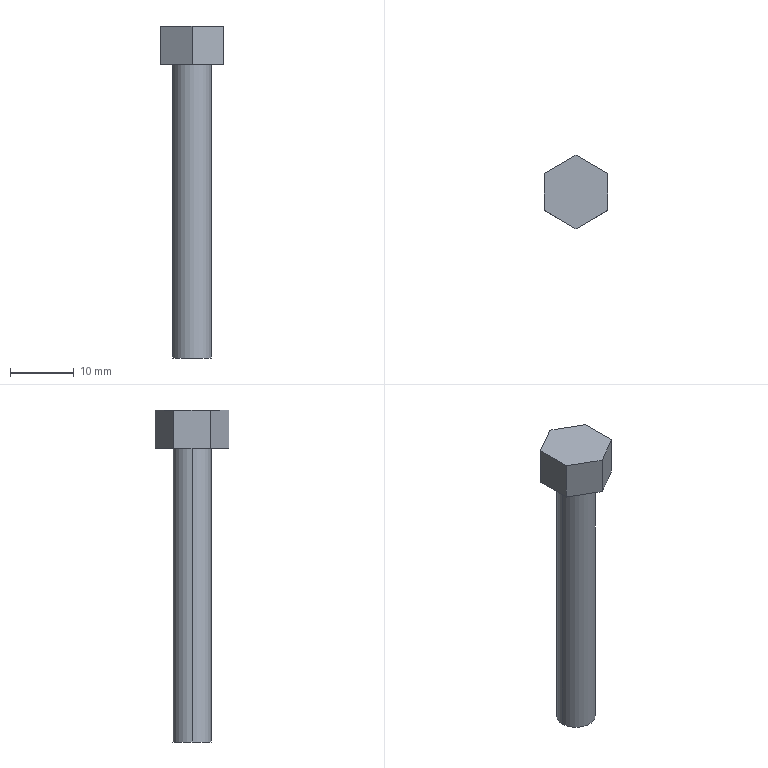Part | STEP file | 11-FG-E00711 | 1 solid | 11 faces | box 10 x 11.547 x 52 mm | volume 1820 mm3 | plane 9 | cylinder 2 | commonest cylinder face diameters 6 x2
STEP:
#1=CARTESIAN_POINT('',(3.,0.,46.));
#2=VERTEX_POINT('',#1);
#3=CARTESIAN_POINT('',(-3.,0.,46.));
#4=VERTEX_POINT('',#3);
#5=CARTESIAN_POINT('',(0.,0.,46.));
#6=DIRECTION('',(0.,0.,1.));
#7=DIRECTION('',(1.,0.,0.));
#8=AXIS2_PLACEMENT_3D('',#5,#6,#7);
#9=CIRCLE('',#8,3.);
#10=EDGE_CURVE('',#2,#4,#9,.T.);
#11=ORIENTED_EDGE('',*,*,#10,.F.);
#12=CARTESIAN_POINT('',(3.,0.,0.));
#13=VERTEX_POINT('',#12);
#14=CARTESIAN_POINT('',(3.,0.,46.));
#15=DIRECTION('',(0.,0.,-1.));
#16=VECTOR('',#15,1000.);
#17=LINE('',#14,#16);
#18=EDGE_CURVE('',#2,#13,#17,.T.);
#19=ORIENTED_EDGE('',*,*,#18,.T.);
#20=CARTESIAN_POINT('',(-3.,0.,0.));
#21=VERTEX_POINT('',#20);
#22=CARTESIAN_POINT('',(0.,0.,0.));
#23=DIRECTION('',(0.,0.,1.));
#24=DIRECTION('',(1.,0.,0.));
#25=AXIS2_PLACEMENT_3D('',#22,#23,#24);
#26=CIRCLE('',#25,3.);
#27=EDGE_CURVE('',#13,#21,#26,.T.);
#28=ORIENTED_EDGE('',*,*,#27,.T.);
#29=CARTESIAN_POINT('',(-3.,0.,46.));
#30=DIRECTION('',(0.,0.,-1.));
#31=VECTOR('',#30,1000.);
#32=LINE('',#29,#31);
#33=EDGE_CURVE('',#4,#21,#32,.T.);
#34=ORIENTED_EDGE('',*,*,#33,.F.);
#35=EDGE_LOOP('',(#11,#19,#28,#34));
#36=FACE_OUTER_BOUND('',#35,.T.);
#37=CARTESIAN_POINT('',(0.,0.,46.));
#38=DIRECTION('',(0.,0.,-1.));
#39=DIRECTION('',(-1.,0.,0.));
#40=AXIS2_PLACEMENT_3D('',#37,#38,#39);
#41=CYLINDRICAL_SURFACE('',#40,3.);
#42=ADVANCED_FACE('',(#36),#41,.T.);
#43=ORIENTED_EDGE('',*,*,#18,.F.);
#44=CARTESIAN_POINT('',(0.,0.,46.));
#45=DIRECTION('',(0.,0.,1.));
#46=DIRECTION('',(1.,0.,0.));
#47=AXIS2_PLACEMENT_3D('',#44,#45,#46);
#48=CIRCLE('',#47,3.);
#49=EDGE_CURVE('',#4,#2,#48,.T.);
#50=ORIENTED_EDGE('',*,*,#49,.F.);
#51=ORIENTED_EDGE('',*,*,#33,.T.);
#52=CARTESIAN_POINT('',(0.,0.,0.));
#53=DIRECTION('',(0.,0.,1.));
#54=DIRECTION('',(1.,0.,0.));
#55=AXIS2_PLACEMENT_3D('',#52,#53,#54);
#56=CIRCLE('',#55,3.);
#57=EDGE_CURVE('',#21,#13,#56,.T.);
#58=ORIENTED_EDGE('',*,*,#57,.T.);
#59=EDGE_LOOP('',(#43,#50,#51,#58));
#60=FACE_OUTER_BOUND('',#59,.T.);
#61=CARTESIAN_POINT('',(0.,0.,46.));
#62=DIRECTION('',(0.,0.,-1.));
#63=DIRECTION('',(-1.,0.,0.));
#64=AXIS2_PLACEMENT_3D('',#61,#62,#63);
#65=CYLINDRICAL_SURFACE('',#64,3.);
#66=ADVANCED_FACE('',(#60),#65,.T.);
#67=ORIENTED_EDGE('',*,*,#57,.F.);
#68=ORIENTED_EDGE('',*,*,#27,.F.);
#69=EDGE_LOOP('',(#67,#68));
#70=FACE_OUTER_BOUND('',#69,.T.);
#71=CARTESIAN_POINT('',(0.,0.,0.));
#72=DIRECTION('',(0.,0.,1.));
#73=DIRECTION('',(1.,0.,0.));
#74=AXIS2_PLACEMENT_3D('',#71,#72,#73);
#75=PLANE('',#74);
#76=ADVANCED_FACE('',(#70),#75,.F.);
#77=CARTESIAN_POINT('',(5.,2.887,46.));
#78=VERTEX_POINT('',#77);
#79=CARTESIAN_POINT('',(0.,5.774,46.));
#80=VERTEX_POINT('',#79);
#81=CARTESIAN_POINT('',(5.,2.887,46.));
#82=DIRECTION('',(-0.866,0.5,0.));
#83=VECTOR('',#82,1000.);
#84=LINE('',#81,#83);
#85=EDGE_CURVE('',#78,#80,#84,.T.);
#86=ORIENTED_EDGE('',*,*,#85,.F.);
#87=CARTESIAN_POINT('',(5.,-2.887,46.));
#88=VERTEX_POINT('',#87);
#89=CARTESIAN_POINT('',(5.,-2.887,46.));
#90=DIRECTION('',(0.,1.,0.));
#91=VECTOR('',#90,1000.);
#92=LINE('',#89,#91);
#93=EDGE_CURVE('',#88,#78,#92,.T.);
#94=ORIENTED_EDGE('',*,*,#93,.F.);
#95=CARTESIAN_POINT('',(0.,-5.774,46.));
#96=VERTEX_POINT('',#95);
#97=CARTESIAN_POINT('',(0.,-5.774,46.));
#98=DIRECTION('',(0.866,0.5,0.));
#99=VECTOR('',#98,1000.);
#100=LINE('',#97,#99);
#101=EDGE_CURVE('',#96,#88,#100,.T.);
#102=ORIENTED_EDGE('',*,*,#101,.F.);
#103=CARTESIAN_POINT('',(-5.,-2.887,46.));
#104=VERTEX_POINT('',#103);
#105=CARTESIAN_POINT('',(-5.,-2.887,46.));
#106=DIRECTION('',(0.866,-0.5,0.));
#107=VECTOR('',#106,1000.);
#108=LINE('',#105,#107);
#109=EDGE_CURVE('',#104,#96,#108,.T.);
#110=ORIENTED_EDGE('',*,*,#109,.F.);
#111=CARTESIAN_POINT('',(-5.,2.887,46.));
#112=VERTEX_POINT('',#111);
#113=CARTESIAN_POINT('',(-5.,2.887,46.));
#114=DIRECTION('',(0.,-1.,0.));
#115=VECTOR('',#114,1000.);
#116=LINE('',#113,#115);
#117=EDGE_CURVE('',#112,#104,#116,.T.);
#118=ORIENTED_EDGE('',*,*,#117,.F.);
#119=CARTESIAN_POINT('',(0.,5.774,46.));
#120=DIRECTION('',(-0.866,-0.5,0.));
#121=VECTOR('',#120,1000.);
#122=LINE('',#119,#121);
#123=EDGE_CURVE('',#80,#112,#122,.T.);
#124=ORIENTED_EDGE('',*,*,#123,.F.);
#125=EDGE_LOOP('',(#86,#94,#102,#110,#118,#124));
#126=FACE_OUTER_BOUND('',#125,.T.);
#127=ORIENTED_EDGE('',*,*,#49,.T.);
#128=ORIENTED_EDGE('',*,*,#10,.T.);
#129=EDGE_LOOP('',(#127,#128));
#130=FACE_BOUND('',#129,.T.);
#131=CARTESIAN_POINT('',(0.,5.774,46.));
#132=DIRECTION('',(0.,0.,1.));
#133=DIRECTION('',(1.,0.,0.));
#134=AXIS2_PLACEMENT_3D('',#131,#132,#133);
#135=PLANE('',#134);
#136=ADVANCED_FACE('',(#126,#130),#135,.F.);
#137=ORIENTED_EDGE('',*,*,#85,.T.);
#138=CARTESIAN_POINT('',(0.,5.774,52.));
#139=VERTEX_POINT('',#138);
#140=CARTESIAN_POINT('',(0.,5.774,52.));
#141=DIRECTION('',(0.,0.,-1.));
#142=VECTOR('',#141,1000.);
#143=LINE('',#140,#142);
#144=EDGE_CURVE('',#139,#80,#143,.T.);
#145=ORIENTED_EDGE('',*,*,#144,.F.);
#146=CARTESIAN_POINT('',(5.,2.887,52.));
#147=VERTEX_POINT('',#146);
#148=CARTESIAN_POINT('',(5.,2.887,52.));
#149=DIRECTION('',(-0.866,0.5,0.));
#150=VECTOR('',#149,1000.);
#151=LINE('',#148,#150);
#152=EDGE_CURVE('',#147,#139,#151,.T.);
#153=ORIENTED_EDGE('',*,*,#152,.F.);
#154=CARTESIAN_POINT('',(5.,2.887,52.));
#155=DIRECTION('',(0.,0.,-1.));
#156=VECTOR('',#155,1000.);
#157=LINE('',#154,#156);
#158=EDGE_CURVE('',#147,#78,#157,.T.);
#159=ORIENTED_EDGE('',*,*,#158,.T.);
#160=EDGE_LOOP('',(#137,#145,#153,#159));
#161=FACE_OUTER_BOUND('',#160,.T.);
#162=CARTESIAN_POINT('',(5.,2.887,52.));
#163=DIRECTION('',(-0.5,-0.866,0.));
#164=DIRECTION('',(0.866,-0.5,0.));
#165=AXIS2_PLACEMENT_3D('',#162,#163,#164);
#166=PLANE('',#165);
#167=ADVANCED_FACE('',(#161),#166,.F.);
#168=ORIENTED_EDGE('',*,*,#123,.T.);
#169=CARTESIAN_POINT('',(-5.,2.887,52.));
#170=VERTEX_POINT('',#169);
#171=CARTESIAN_POINT('',(-5.,2.887,52.));
#172=DIRECTION('',(0.,0.,-1.));
#173=VECTOR('',#172,1000.);
#174=LINE('',#171,#173);
#175=EDGE_CURVE('',#170,#112,#174,.T.);
#176=ORIENTED_EDGE('',*,*,#175,.F.);
#177=CARTESIAN_POINT('',(0.,5.774,52.));
#178=DIRECTION('',(-0.866,-0.5,0.));
#179=VECTOR('',#178,1000.);
#180=LINE('',#177,#179);
#181=EDGE_CURVE('',#139,#170,#180,.T.);
#182=ORIENTED_EDGE('',*,*,#181,.F.);
#183=ORIENTED_EDGE('',*,*,#144,.T.);
#184=EDGE_LOOP('',(#168,#176,#182,#183));
#185=FACE_OUTER_BOUND('',#184,.T.);
#186=CARTESIAN_POINT('',(0.,5.774,52.));
#187=DIRECTION('',(0.5,-0.866,0.));
#188=DIRECTION('',(0.866,0.5,0.));
#189=AXIS2_PLACEMENT_3D('',#186,#187,#188);
#190=PLANE('',#189);
#191=ADVANCED_FACE('',(#185),#190,.F.);
#192=ORIENTED_EDGE('',*,*,#117,.T.);
#193=CARTESIAN_POINT('',(-5.,-2.887,52.));
#194=VERTEX_POINT('',#193);
#195=CARTESIAN_POINT('',(-5.,-2.887,52.));
#196=DIRECTION('',(0.,0.,-1.));
#197=VECTOR('',#196,1000.);
#198=LINE('',#195,#197);
#199=EDGE_CURVE('',#194,#104,#198,.T.);
#200=ORIENTED_EDGE('',*,*,#199,.F.);
#201=CARTESIAN_POINT('',(-5.,2.887,52.));
#202=DIRECTION('',(0.,-1.,0.));
#203=VECTOR('',#202,1000.);
#204=LINE('',#201,#203);
#205=EDGE_CURVE('',#170,#194,#204,.T.);
#206=ORIENTED_EDGE('',*,*,#205,.F.);
#207=ORIENTED_EDGE('',*,*,#175,.T.);
#208=EDGE_LOOP('',(#192,#200,#206,#207));
#209=FACE_OUTER_BOUND('',#208,.T.);
#210=CARTESIAN_POINT('',(-5.,2.887,52.));
#211=DIRECTION('',(1.,0.,0.));
#212=DIRECTION('',(0.,0.,-1.));
#213=AXIS2_PLACEMENT_3D('',#210,#211,#212);
#214=PLANE('',#213);
#215=ADVANCED_FACE('',(#209),#214,.F.);
#216=ORIENTED_EDGE('',*,*,#109,.T.);
#217=CARTESIAN_POINT('',(0.,-5.774,52.));
#218=VERTEX_POINT('',#217);
#219=CARTESIAN_POINT('',(0.,-5.774,52.));
#220=DIRECTION('',(0.,0.,-1.));
#221=VECTOR('',#220,1000.);
#222=LINE('',#219,#221);
#223=EDGE_CURVE('',#218,#96,#222,.T.);
#224=ORIENTED_EDGE('',*,*,#223,.F.);
#225=CARTESIAN_POINT('',(-5.,-2.887,52.));
#226=DIRECTION('',(0.866,-0.5,0.));
#227=VECTOR('',#226,1000.);
#228=LINE('',#225,#227);
#229=EDGE_CURVE('',#194,#218,#228,.T.);
#230=ORIENTED_EDGE('',*,*,#229,.F.);
#231=ORIENTED_EDGE('',*,*,#199,.T.);
#232=EDGE_LOOP('',(#216,#224,#230,#231));
#233=FACE_OUTER_BOUND('',#232,.T.);
#234=CARTESIAN_POINT('',(-5.,-2.887,52.));
#235=DIRECTION('',(0.5,0.866,0.));
#236=DIRECTION('',(-0.866,0.5,0.));
#237=AXIS2_PLACEMENT_3D('',#234,#235,#236);
#238=PLANE('',#237);
#239=ADVANCED_FACE('',(#233),#238,.F.);
#240=ORIENTED_EDGE('',*,*,#101,.T.);
#241=CARTESIAN_POINT('',(5.,-2.887,52.));
#242=VERTEX_POINT('',#241);
#243=CARTESIAN_POINT('',(5.,-2.887,52.));
#244=DIRECTION('',(0.,0.,-1.));
#245=VECTOR('',#244,1000.);
#246=LINE('',#243,#245);
#247=EDGE_CURVE('',#242,#88,#246,.T.);
#248=ORIENTED_EDGE('',*,*,#247,.F.);
#249=CARTESIAN_POINT('',(0.,-5.774,52.));
#250=DIRECTION('',(0.866,0.5,0.));
#251=VECTOR('',#250,1000.);
#252=LINE('',#249,#251);
#253=EDGE_CURVE('',#218,#242,#252,.T.);
#254=ORIENTED_EDGE('',*,*,#253,.F.);
#255=ORIENTED_EDGE('',*,*,#223,.T.);
#256=EDGE_LOOP('',(#240,#248,#254,#255));
#257=FACE_OUTER_BOUND('',#256,.T.);
#258=CARTESIAN_POINT('',(0.,-5.774,52.));
#259=DIRECTION('',(-0.5,0.866,0.));
#260=DIRECTION('',(-0.866,-0.5,0.));
#261=AXIS2_PLACEMENT_3D('',#258,#259,#260);
#262=PLANE('',#261);
#263=ADVANCED_FACE('',(#257),#262,.F.);
#264=ORIENTED_EDGE('',*,*,#93,.T.);
#265=ORIENTED_EDGE('',*,*,#158,.F.);
#266=CARTESIAN_POINT('',(5.,-2.887,52.));
#267=DIRECTION('',(0.,1.,0.));
#268=VECTOR('',#267,1000.);
#269=LINE('',#266,#268);
#270=EDGE_CURVE('',#242,#147,#269,.T.);
#271=ORIENTED_EDGE('',*,*,#270,.F.);
#272=ORIENTED_EDGE('',*,*,#247,.T.);
#273=EDGE_LOOP('',(#264,#265,#271,#272));
#274=FACE_OUTER_BOUND('',#273,.T.);
#275=CARTESIAN_POINT('',(5.,-2.887,52.));
#276=DIRECTION('',(-1.,0.,0.));
#277=DIRECTION('',(0.,-1.,0.));
#278=AXIS2_PLACEMENT_3D('',#275,#276,#277);
#279=PLANE('',#278);
#280=ADVANCED_FACE('',(#274),#279,.F.);
#281=ORIENTED_EDGE('',*,*,#152,.T.);
#282=ORIENTED_EDGE('',*,*,#181,.T.);
#283=ORIENTED_EDGE('',*,*,#205,.T.);
#284=ORIENTED_EDGE('',*,*,#229,.T.);
#285=ORIENTED_EDGE('',*,*,#253,.T.);
#286=ORIENTED_EDGE('',*,*,#270,.T.);
#287=EDGE_LOOP('',(#281,#282,#283,#284,#285,#286));
#288=FACE_OUTER_BOUND('',#287,.T.);
#289=CARTESIAN_POINT('',(0.,5.774,52.));
#290=DIRECTION('',(0.,0.,1.));
#291=DIRECTION('',(1.,0.,0.));
#292=AXIS2_PLACEMENT_3D('',#289,#290,#291);
#293=PLANE('',#292);
#294=ADVANCED_FACE('',(#288),#293,.T.);
#295=CLOSED_SHELL('',(#42,#66,#76,#136,#167,#191,#215,#239,#263,#280,#294));
#296=MANIFOLD_SOLID_BREP('',#295);
#297=CARTESIAN_POINT('',(0.,0.,0.));
#298=DIRECTION('',(0.,0.,1.));
#299=DIRECTION('',(1.,0.,0.));
#300=AXIS2_PLACEMENT_3D('',#297,#298,#299);
#301=(LENGTH_UNIT()NAMED_UNIT(*)SI_UNIT(.MILLI.,.METRE.));
#302=UNCERTAINTY_MEASURE_WITH_UNIT(LENGTH_MEASURE(0.00001),#301,'','');
#303=(NAMED_UNIT(*)PLANE_ANGLE_UNIT()SI_UNIT($,.RADIAN.));
#304=(NAMED_UNIT(*)SI_UNIT($,.STERADIAN.)SOLID_ANGLE_UNIT());
#305=(GEOMETRIC_REPRESENTATION_CONTEXT(3)GLOBAL_UNCERTAINTY_ASSIGNED_CONTEXT((#302))GLOBAL_UNIT_ASSIGNED_CONTEXT((#301,#303,#304))REPRESENTATION_CONTEXT('',''));
#306=ADVANCED_BREP_SHAPE_REPRESENTATION('',(#296,#300),#305);